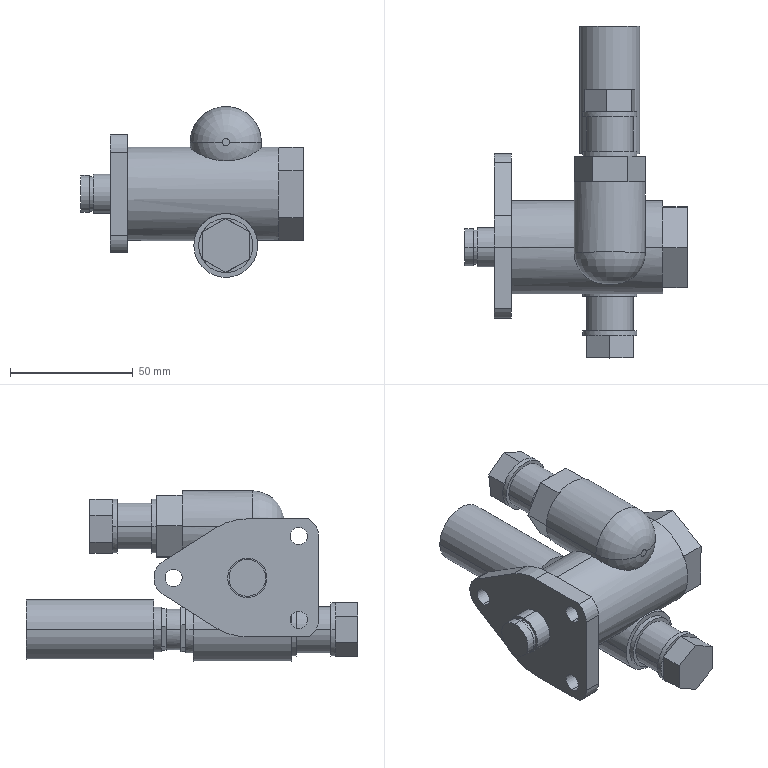Part | SolidWorks | features BaseBody 1 | 1 solid | 153 faces | box 90.5 x 135 x 69.5 mm | volume 184767 mm3 | plane 108 | cylinder 43 | torus 2 | commonest cylinder face diameters 22 x8 7 x6 19 x6 16 x5 14 x2 15 x2